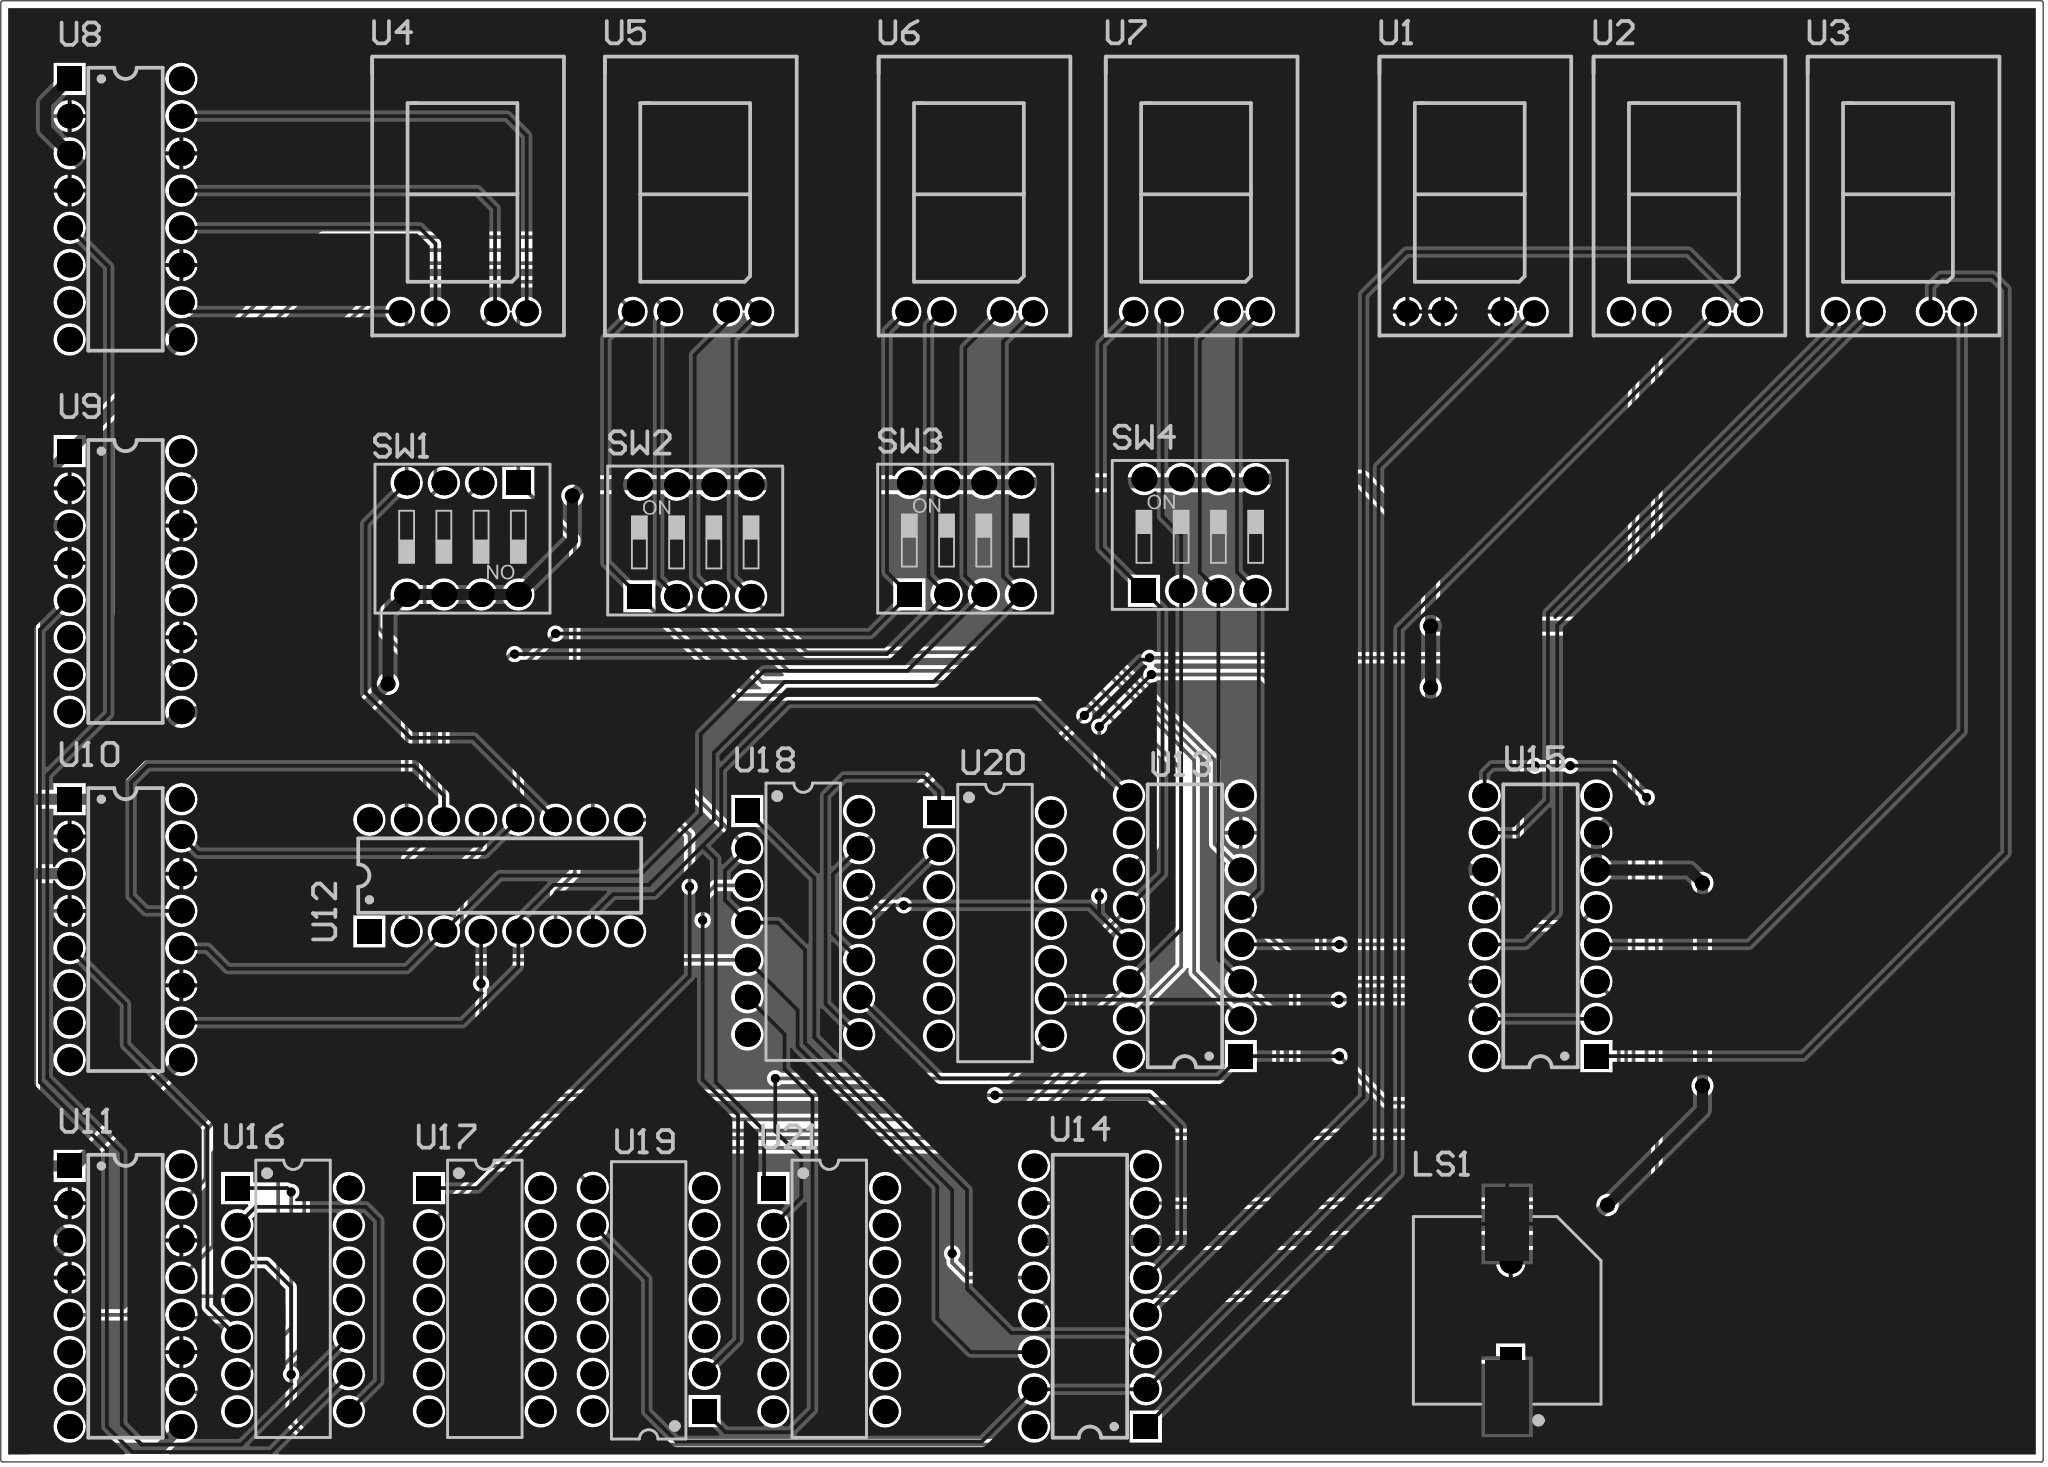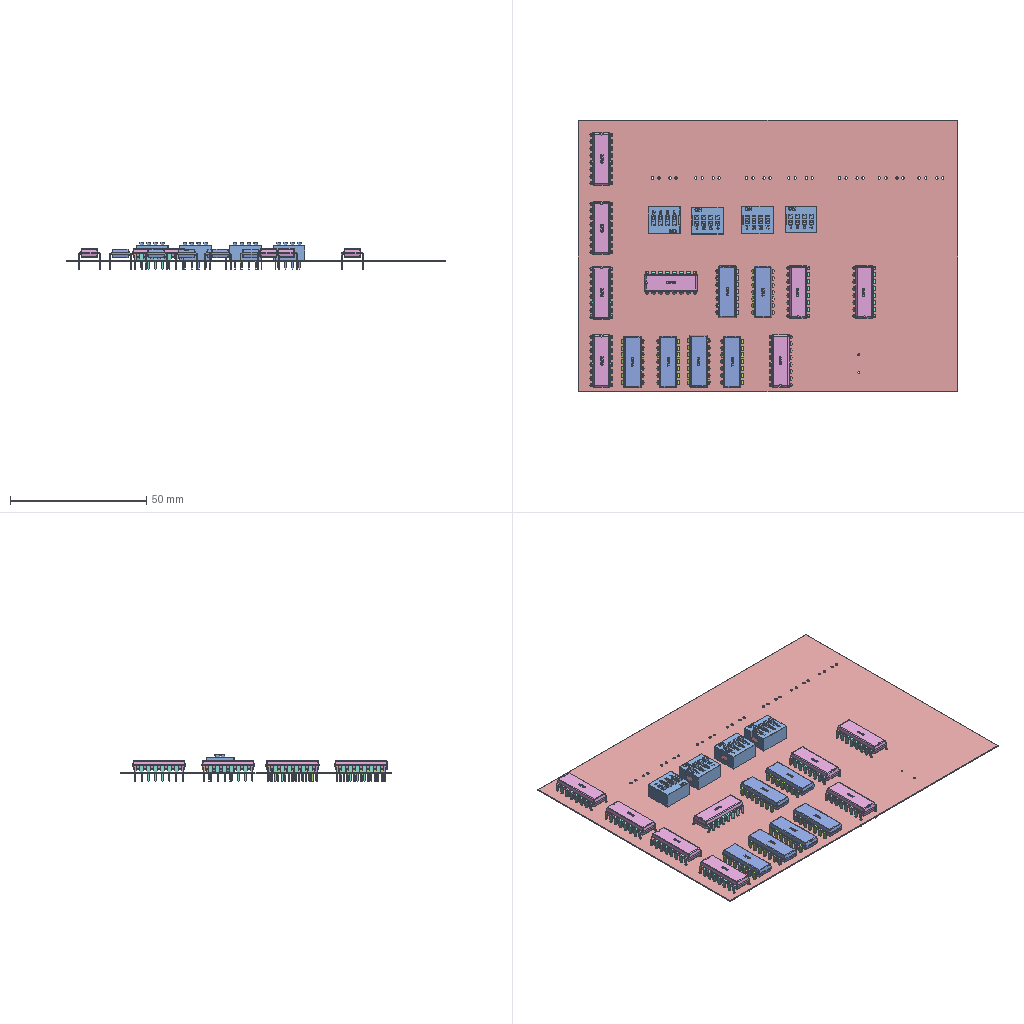Circuit board layout | Altium Designer | box 139.3 x 99.7 x 10 mm
Layer stack:
# Altium Designer layer stack of  (unit mm; dielectric type: 0 none, 1 core, 2 prepreg, 3 surface material)
index,name,kind,layer,copper_thickness_mm,dielectric_type,dielectric_thickness_mm,dielectric_material,dielectric_constant
0,Top Paste,other,,,,,,
1,Top Overlay,other,,,,,,
2,Top Solder,dielectric,,,3,0.0102,Solder Resist,3.5
3,Top Layer,copper,Top Layer,0.0356,,,,
4,Dielectric 1,dielectric,,,0,0.32,FR-4,4.8
5,Bottom Layer,copper,Bottom Layer,0.0356,,,,
6,Bottom Solder,dielectric,,,3,0.0102,Solder Resist,3.5
7,Bottom Overlay,other,,,,,,
8,Bottom Paste,other,,,,,,
# drill layer pairs: low layer,high layer
drill_pair,Top Layer,Bottom Layer
Part placement:
Designator,Comment,Layer,Footprint,Center-X(mm),Center-Y(mm),Rotation
U21,74LS04,TopLayer,DIP14,89.408,62.625,360
U20,MC14023UBCL,TopLayer,DIP14,100.711,88.265,360
U19,MC14023UBCL,TopLayer,DIP14,77.089,62.648,180
U18,74LS00,TopLayer,DIP14,87.63,88.355,360
U17,74LS04,TopLayer,DIP14,65.913,62.625,360
U16,74LS32,TopLayer,DIP14,52.832,62.625,360
U15,74HC283D,TopLayer,DIP16,137.922,88.138,180
U14,74HC283D,TopLayer,DIP16,107.188,62.865,180
U13,74HC283D,TopLayer,DIP16,113.665,88.138,180
U12,74HC283D,TopLayer,DIP16,66.929,91.567,90
U11,SN74LS85N,TopLayer,DIP16,41.402,62.865,0
U10,SN74LS85N,TopLayer,DIP16,41.402,87.884,0
U9,SN74LS85N,TopLayer,DIP16,41.402,111.633,0
U8,SN74LS85N,TopLayer,DIP16,41.402,137.033,360
U7,LCD1,TopLayer,DCD-HEX,114.49,130.048,0
U6,LCD1,TopLayer,DCD-HEX,98.996,130.048,0
U5,LCD1,TopLayer,DCD-HEX,80.328,130.048,0
U4,LCD1,TopLayer,DCD-HEX,64.453,130.048,0
U3,LCD1,TopLayer,DCD-HEX,162.369,130.048,0
U2,LCD1,TopLayer,DCD-HEX,147.764,130.048,0
U1,LCD1,TopLayer,DCD-HEX,133.16,130.048,0
SW4,SW-4P,TopLayer,CSW_DIP-4P,114.681,114.808,0
SW3,SW-4P,TopLayer,CSW_DIP-4P,98.679,114.554,0
SW2,SW-4P,TopLayer,CSW_DIP-4P,80.264,114.427,360
SW1,SW-4P,TopLayer,CSW_DIP-4P,64.389,114.554,180
LS1,Buzzer,TopLayer,ABSM-1574,135.77,61.901,90
Pad and via stacks:
# Altium Designer via and pad stacks of  (unit mm). Each distinct definition once, with the count of objects using it.
# via: kind,start_layer,end_layer,hole_mm,diameter_mm,mode(0 simple;1 top-mid-bottom;2 full stack),diameter_per_layer,count,example_net
# pad: kind,layer,hole_mm,hole_type(0 round;1 square;2 slot),plating,top_size,top_shape(1 round;2 rect;3 octagon;9 rounded rect),mid_size,bottom_size,mode,footprint,size_per_layer,count,example
pad,Top Layer,0,0,plated,3x5,2,3x5,3x5,0,ABSM-1574,,2,LS1.1
pad,Multi-Layer,0.8,0,plated,1.7x1.7,1,1.7x1.7,1.7x1.7,0,DIP16,,120,U15.16
pad,Multi-Layer,0.8,0,plated,1.7x1.7,2,1.7x1.7,1.7x1.7,0,DIP16,,8,U15.1
pad,Multi-Layer,0.9144,0,plated,1.524x1.524,1,1.524x1.524,1.524x1.524,0,DCD-HEX,,28,U3.3
pad,Multi-Layer,0.9,0,plated,1.7x1.7,1,1.7x1.7,1.7x1.7,0,CSW DIP-4P,,28,SW4.5
pad,Multi-Layer,0.9,0,plated,1.7x1.7,2,1.7x1.7,1.7x1.7,0,CSW DIP-4P,,4,SW4.1
pad,Multi-Layer,0.8,0,plated,1.7x1.7,2,1.7x1.7,1.7x1.7,0,DIP14,,6,U16.1
pad,Multi-Layer,0.8,0,plated,1.7x1.7,1,1.7x1.7,1.7x1.7,0,DIP14,,78,U16.2
pad,Multi-Layer,0.7,0,plated,1.5x1.5,2,1.5x1.5,1.5x1.5,0,ABSM-1574,,1,LS1.1A
pad,Multi-Layer,0.7,0,plated,1.5x1.5,1,1.5x1.5,1.5x1.5,0,ABSM-1574,,1,LS1.2A
via,Top Layer,Bottom Layer,0.3048,0.6096,0,,22,NetU14_7
via,Top Layer,Bottom Layer,0.508,1.016,0,,7,+5
Copper pours:
name,layer,net,type(0 solid;1 hatched;2 none)
G,Bottom Layer,GND,0
G,Top Layer,GND,0
Design rules, without the lines most boards share:
# Altium Designer design rules of  (exported by Altium Designer, unit mm)
# columns: name | kind | enabled | priority | scope1 | scope2 | descriptor | typed fields (field=value)
SilkToSilkClearance | 55 | enabled | 1 | All | All | Silk to Silk (Clearance=0mil) (All),(All) |
SilkToSolderMaskClearance | 54 | enabled | 1 | IsPad | All | Silk To Solder Mask (Clearance=0mil) (IsPad),(All) |
MinimumSolderMaskSliver | 53 | enabled | 1 | All | All | Minimum Solder Mask Sliver (Gap=0mil) (All),(All) |
HoleToHoleClearance | 52 | enabled | 1 | All | All | Hole To Hole Clearance (Gap=10mil) (All),(All) | gap=0.254
DiffPairsRouting | 51 | enabled | 1 | All | All | Differential Pairs Uncoupled Length using the Gap Constraints (Min=10mil) (Max=10mil) (Prefered=10mil)  and Width Constraints (Min=15mil) (Max=15mil) (Prefered=15mil) (All) |
SolderMaskExpansion | 13 | enabled | 1 | All | All | Solder Mask Expansion (Expansion =4mil) (All) | expansion=0.1016
PasteMaskExpansion | 14 | enabled | 1 | All | All | Paste Mask Expansion (Expansion =0mil) (All) | expansion=0
RoutingVias | 11 | enabled | 1 | All | All | Routing Via (MinHoleWidth=28mil) (MaxHoleWidth=28mil) (PreferredHoleWidth=28mil) (MinWidth=50mil) (MaxWidth=50mil) (PreferedWidth=50mil) (All) | via_min_hole=0.7112 via_max_hole=0.7112 via_preferred_diameter=1.27 via_preferred_hole=0.7112
Width | 2 | enabled | 1 | All | All | Width Constraint (Min=10mil) (Max=13110.236mil) (Preferred=10mil) (All) |
PolygonConnect | 20 | enabled | 1 | All | All | Polygon Connect Rule(Relief Connect )(Conductor Width=10mil) (Relief Angle=90 Angle) (Entries=4) (Air Gap Width=10mil) (All),(All) | connect_style(0=relief,1=direct,2=none)=0 relief_conductor_width=0.254 relief_entries=4
PlaneConnect | 6 | enabled | 1 | All | All | Power Plane Connect Rule(Relief Connect )(Expansion=20mil) (Conductor Width=10mil) (Air Gap=10mil) (Entries=4) (All) | relief_conductor_width=0.254 relief_entries=4 relief_expansion=0.508
Clearance | 0 | enabled | 1 | All | All | Clearance Constraint (Gap=10mil) (All),(All) | gap=0.254
Classes set for this board:
# Altium Designer classes of  (member kind: 0 net, 1 component, 2 from-to, 3 pad, 4 layer, 5 differential pair, 6 design channel, 7 polygon, 8 structure, 9 xSignal)
# columns: class name | member kind | superclass | members
Sheet1 | 1 | no | LS1; SW1; SW2; SW3; SW4; U1; U2; U3; U4; U5; U6; U7; U8; U9; U10; U11; U12; U13; U14; U15; U16; U17; U18; U19; U20; U21;